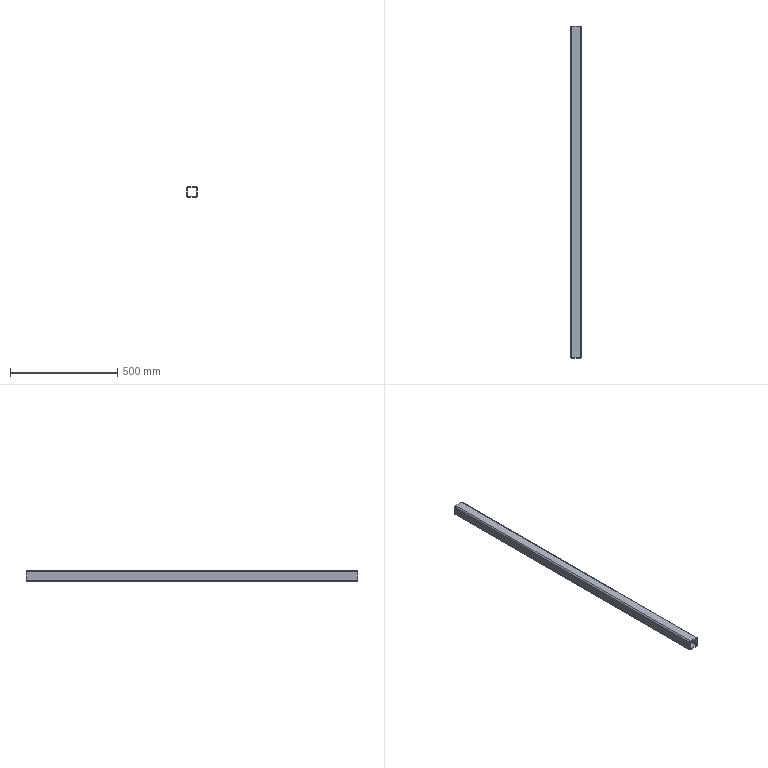Part | SolidWorks | features Extrusion 1 | 1 solid | 18 faces | box 50 x 1550 x 50 mm | volume 1348431 mm3 | plane 10 | cylinder 8 | commonest cylinder face diameters 2 x4 12 x4
STEP:
#1=CARTESIAN_POINT('',(-25.,1550.,19.));
#2=VERTEX_POINT('',#1);
#3=CARTESIAN_POINT('',(-19.,1550.,25.));
#4=VERTEX_POINT('',#3);
#5=CARTESIAN_POINT('',(-19.,1550.,19.));
#6=DIRECTION('',(0.,1.,0.));
#7=DIRECTION('',(0.,0.,-1.));
#8=AXIS2_PLACEMENT_3D('',#5,#6,#7);
#9=CIRCLE('',#8,6.);
#10=EDGE_CURVE('',#2,#4,#9,.T.);
#11=ORIENTED_EDGE('',*,*,#10,.T.);
#12=CARTESIAN_POINT('',(19.,1550.,25.));
#13=VERTEX_POINT('',#12);
#14=CARTESIAN_POINT('',(-19.,1550.,25.));
#15=DIRECTION('',(1.,0.,0.));
#16=VECTOR('',#15,1000.);
#17=LINE('',#14,#16);
#18=EDGE_CURVE('',#4,#13,#17,.T.);
#19=ORIENTED_EDGE('',*,*,#18,.T.);
#20=CARTESIAN_POINT('',(25.,1550.,19.));
#21=VERTEX_POINT('',#20);
#22=CARTESIAN_POINT('',(19.,1550.,19.));
#23=DIRECTION('',(0.,1.,0.));
#24=DIRECTION('',(0.,0.,1.));
#25=AXIS2_PLACEMENT_3D('',#22,#23,#24);
#26=CIRCLE('',#25,6.);
#27=EDGE_CURVE('',#13,#21,#26,.T.);
#28=ORIENTED_EDGE('',*,*,#27,.T.);
#29=CARTESIAN_POINT('',(25.,1550.,-19.));
#30=VERTEX_POINT('',#29);
#31=CARTESIAN_POINT('',(25.,1550.,19.));
#32=DIRECTION('',(0.,0.,-1.));
#33=VECTOR('',#32,1000.);
#34=LINE('',#31,#33);
#35=EDGE_CURVE('',#21,#30,#34,.T.);
#36=ORIENTED_EDGE('',*,*,#35,.T.);
#37=CARTESIAN_POINT('',(19.,1550.,-25.));
#38=VERTEX_POINT('',#37);
#39=CARTESIAN_POINT('',(19.,1550.,-19.));
#40=DIRECTION('',(0.,1.,0.));
#41=DIRECTION('',(0.,0.,-1.));
#42=AXIS2_PLACEMENT_3D('',#39,#40,#41);
#43=CIRCLE('',#42,6.);
#44=EDGE_CURVE('',#30,#38,#43,.T.);
#45=ORIENTED_EDGE('',*,*,#44,.T.);
#46=CARTESIAN_POINT('',(-19.,1550.,-25.));
#47=VERTEX_POINT('',#46);
#48=CARTESIAN_POINT('',(-19.,1550.,-25.));
#49=DIRECTION('',(-1.,0.,0.));
#50=VECTOR('',#49,1000.);
#51=LINE('',#48,#50);
#52=EDGE_CURVE('',#38,#47,#51,.T.);
#53=ORIENTED_EDGE('',*,*,#52,.T.);
#54=CARTESIAN_POINT('',(-25.,1550.,-19.));
#55=VERTEX_POINT('',#54);
#56=CARTESIAN_POINT('',(-19.,1550.,-19.));
#57=DIRECTION('',(0.,1.,0.));
#58=DIRECTION('',(0.,0.,-1.));
#59=AXIS2_PLACEMENT_3D('',#56,#57,#58);
#60=CIRCLE('',#59,6.);
#61=EDGE_CURVE('',#47,#55,#60,.T.);
#62=ORIENTED_EDGE('',*,*,#61,.T.);
#63=CARTESIAN_POINT('',(-25.,1550.,19.));
#64=DIRECTION('',(0.,0.,1.));
#65=VECTOR('',#64,1000.);
#66=LINE('',#63,#65);
#67=EDGE_CURVE('',#55,#2,#66,.T.);
#68=ORIENTED_EDGE('',*,*,#67,.T.);
#69=EDGE_LOOP('',(#11,#19,#28,#36,#45,#53,#62,#68));
#70=FACE_OUTER_BOUND('',#69,.T.);
#71=CARTESIAN_POINT('',(-20.,1550.,19.));
#72=VERTEX_POINT('',#71);
#73=CARTESIAN_POINT('',(-19.,1550.,20.));
#74=VERTEX_POINT('',#73);
#75=CARTESIAN_POINT('',(-19.,1550.,19.));
#76=DIRECTION('',(0.,1.,0.));
#77=DIRECTION('',(0.,0.,-1.));
#78=AXIS2_PLACEMENT_3D('',#75,#76,#77);
#79=CIRCLE('',#78,1.);
#80=EDGE_CURVE('',#72,#74,#79,.T.);
#81=ORIENTED_EDGE('',*,*,#80,.F.);
#82=CARTESIAN_POINT('',(-20.,1550.,-19.));
#83=VERTEX_POINT('',#82);
#84=CARTESIAN_POINT('',(-20.,1550.,19.));
#85=DIRECTION('',(0.,0.,1.));
#86=VECTOR('',#85,1000.);
#87=LINE('',#84,#86);
#88=EDGE_CURVE('',#83,#72,#87,.T.);
#89=ORIENTED_EDGE('',*,*,#88,.F.);
#90=CARTESIAN_POINT('',(-19.,1550.,-20.));
#91=VERTEX_POINT('',#90);
#92=CARTESIAN_POINT('',(-19.,1550.,-19.));
#93=DIRECTION('',(0.,1.,0.));
#94=DIRECTION('',(0.,0.,-1.));
#95=AXIS2_PLACEMENT_3D('',#92,#93,#94);
#96=CIRCLE('',#95,1.);
#97=EDGE_CURVE('',#91,#83,#96,.T.);
#98=ORIENTED_EDGE('',*,*,#97,.F.);
#99=CARTESIAN_POINT('',(19.,1550.,-20.));
#100=VERTEX_POINT('',#99);
#101=CARTESIAN_POINT('',(-19.,1550.,-20.));
#102=DIRECTION('',(-1.,0.,0.));
#103=VECTOR('',#102,1000.);
#104=LINE('',#101,#103);
#105=EDGE_CURVE('',#100,#91,#104,.T.);
#106=ORIENTED_EDGE('',*,*,#105,.F.);
#107=CARTESIAN_POINT('',(20.,1550.,-19.));
#108=VERTEX_POINT('',#107);
#109=CARTESIAN_POINT('',(19.,1550.,-19.));
#110=DIRECTION('',(0.,1.,0.));
#111=DIRECTION('',(0.,0.,-1.));
#112=AXIS2_PLACEMENT_3D('',#109,#110,#111);
#113=CIRCLE('',#112,1.);
#114=EDGE_CURVE('',#108,#100,#113,.T.);
#115=ORIENTED_EDGE('',*,*,#114,.F.);
#116=CARTESIAN_POINT('',(20.,1550.,19.));
#117=VERTEX_POINT('',#116);
#118=CARTESIAN_POINT('',(20.,1550.,19.));
#119=DIRECTION('',(0.,0.,-1.));
#120=VECTOR('',#119,1000.);
#121=LINE('',#118,#120);
#122=EDGE_CURVE('',#117,#108,#121,.T.);
#123=ORIENTED_EDGE('',*,*,#122,.F.);
#124=CARTESIAN_POINT('',(19.,1550.,20.));
#125=VERTEX_POINT('',#124);
#126=CARTESIAN_POINT('',(19.,1550.,19.));
#127=DIRECTION('',(0.,1.,0.));
#128=DIRECTION('',(0.,0.,1.));
#129=AXIS2_PLACEMENT_3D('',#126,#127,#128);
#130=CIRCLE('',#129,1.);
#131=EDGE_CURVE('',#125,#117,#130,.T.);
#132=ORIENTED_EDGE('',*,*,#131,.F.);
#133=CARTESIAN_POINT('',(-19.,1550.,20.));
#134=DIRECTION('',(1.,0.,0.));
#135=VECTOR('',#134,1000.);
#136=LINE('',#133,#135);
#137=EDGE_CURVE('',#74,#125,#136,.T.);
#138=ORIENTED_EDGE('',*,*,#137,.F.);
#139=EDGE_LOOP('',(#81,#89,#98,#106,#115,#123,#132,#138));
#140=FACE_BOUND('',#139,.T.);
#141=CARTESIAN_POINT('',(-19.,1550.,19.));
#142=DIRECTION('',(0.,-1.,0.));
#143=DIRECTION('',(0.,0.,-1.));
#144=AXIS2_PLACEMENT_3D('',#141,#142,#143);
#145=PLANE('',#144);
#146=ADVANCED_FACE('',(#70,#140),#145,.F.);
#147=CARTESIAN_POINT('',(-25.,0.,19.));
#148=VERTEX_POINT('',#147);
#149=CARTESIAN_POINT('',(-19.,0.,25.));
#150=VERTEX_POINT('',#149);
#151=CARTESIAN_POINT('',(-19.,0.,19.));
#152=DIRECTION('',(0.,1.,0.));
#153=DIRECTION('',(0.,0.,-1.));
#154=AXIS2_PLACEMENT_3D('',#151,#152,#153);
#155=CIRCLE('',#154,6.);
#156=EDGE_CURVE('',#148,#150,#155,.T.);
#157=ORIENTED_EDGE('',*,*,#156,.F.);
#158=CARTESIAN_POINT('',(-25.,0.,-19.));
#159=VERTEX_POINT('',#158);
#160=CARTESIAN_POINT('',(-25.,0.,19.));
#161=DIRECTION('',(0.,0.,1.));
#162=VECTOR('',#161,1000.);
#163=LINE('',#160,#162);
#164=EDGE_CURVE('',#159,#148,#163,.T.);
#165=ORIENTED_EDGE('',*,*,#164,.F.);
#166=CARTESIAN_POINT('',(-19.,0.,-25.));
#167=VERTEX_POINT('',#166);
#168=CARTESIAN_POINT('',(-19.,0.,-19.));
#169=DIRECTION('',(0.,1.,0.));
#170=DIRECTION('',(0.,0.,-1.));
#171=AXIS2_PLACEMENT_3D('',#168,#169,#170);
#172=CIRCLE('',#171,6.);
#173=EDGE_CURVE('',#167,#159,#172,.T.);
#174=ORIENTED_EDGE('',*,*,#173,.F.);
#175=CARTESIAN_POINT('',(19.,0.,-25.));
#176=VERTEX_POINT('',#175);
#177=CARTESIAN_POINT('',(-19.,0.,-25.));
#178=DIRECTION('',(-1.,0.,0.));
#179=VECTOR('',#178,1000.);
#180=LINE('',#177,#179);
#181=EDGE_CURVE('',#176,#167,#180,.T.);
#182=ORIENTED_EDGE('',*,*,#181,.F.);
#183=CARTESIAN_POINT('',(25.,0.,-19.));
#184=VERTEX_POINT('',#183);
#185=CARTESIAN_POINT('',(19.,0.,-19.));
#186=DIRECTION('',(0.,1.,0.));
#187=DIRECTION('',(0.,0.,-1.));
#188=AXIS2_PLACEMENT_3D('',#185,#186,#187);
#189=CIRCLE('',#188,6.);
#190=EDGE_CURVE('',#184,#176,#189,.T.);
#191=ORIENTED_EDGE('',*,*,#190,.F.);
#192=CARTESIAN_POINT('',(25.,0.,19.));
#193=VERTEX_POINT('',#192);
#194=CARTESIAN_POINT('',(25.,0.,19.));
#195=DIRECTION('',(0.,0.,-1.));
#196=VECTOR('',#195,1000.);
#197=LINE('',#194,#196);
#198=EDGE_CURVE('',#193,#184,#197,.T.);
#199=ORIENTED_EDGE('',*,*,#198,.F.);
#200=CARTESIAN_POINT('',(19.,0.,25.));
#201=VERTEX_POINT('',#200);
#202=CARTESIAN_POINT('',(19.,0.,19.));
#203=DIRECTION('',(0.,1.,0.));
#204=DIRECTION('',(0.,0.,1.));
#205=AXIS2_PLACEMENT_3D('',#202,#203,#204);
#206=CIRCLE('',#205,6.);
#207=EDGE_CURVE('',#201,#193,#206,.T.);
#208=ORIENTED_EDGE('',*,*,#207,.F.);
#209=CARTESIAN_POINT('',(-19.,0.,25.));
#210=DIRECTION('',(1.,0.,0.));
#211=VECTOR('',#210,1000.);
#212=LINE('',#209,#211);
#213=EDGE_CURVE('',#150,#201,#212,.T.);
#214=ORIENTED_EDGE('',*,*,#213,.F.);
#215=EDGE_LOOP('',(#157,#165,#174,#182,#191,#199,#208,#214));
#216=FACE_OUTER_BOUND('',#215,.T.);
#217=CARTESIAN_POINT('',(-20.,0.,-19.));
#218=VERTEX_POINT('',#217);
#219=CARTESIAN_POINT('',(-20.,0.,19.));
#220=VERTEX_POINT('',#219);
#221=CARTESIAN_POINT('',(-20.,0.,19.));
#222=DIRECTION('',(0.,0.,1.));
#223=VECTOR('',#222,1000.);
#224=LINE('',#221,#223);
#225=EDGE_CURVE('',#218,#220,#224,.T.);
#226=ORIENTED_EDGE('',*,*,#225,.T.);
#227=CARTESIAN_POINT('',(-19.,0.,20.));
#228=VERTEX_POINT('',#227);
#229=CARTESIAN_POINT('',(-19.,0.,19.));
#230=DIRECTION('',(0.,1.,0.));
#231=DIRECTION('',(0.,0.,-1.));
#232=AXIS2_PLACEMENT_3D('',#229,#230,#231);
#233=CIRCLE('',#232,1.);
#234=EDGE_CURVE('',#220,#228,#233,.T.);
#235=ORIENTED_EDGE('',*,*,#234,.T.);
#236=CARTESIAN_POINT('',(19.,0.,20.));
#237=VERTEX_POINT('',#236);
#238=CARTESIAN_POINT('',(-19.,0.,20.));
#239=DIRECTION('',(1.,0.,0.));
#240=VECTOR('',#239,1000.);
#241=LINE('',#238,#240);
#242=EDGE_CURVE('',#228,#237,#241,.T.);
#243=ORIENTED_EDGE('',*,*,#242,.T.);
#244=CARTESIAN_POINT('',(20.,0.,19.));
#245=VERTEX_POINT('',#244);
#246=CARTESIAN_POINT('',(19.,0.,19.));
#247=DIRECTION('',(0.,1.,0.));
#248=DIRECTION('',(0.,0.,1.));
#249=AXIS2_PLACEMENT_3D('',#246,#247,#248);
#250=CIRCLE('',#249,1.);
#251=EDGE_CURVE('',#237,#245,#250,.T.);
#252=ORIENTED_EDGE('',*,*,#251,.T.);
#253=CARTESIAN_POINT('',(20.,0.,-19.));
#254=VERTEX_POINT('',#253);
#255=CARTESIAN_POINT('',(20.,0.,19.));
#256=DIRECTION('',(0.,0.,-1.));
#257=VECTOR('',#256,1000.);
#258=LINE('',#255,#257);
#259=EDGE_CURVE('',#245,#254,#258,.T.);
#260=ORIENTED_EDGE('',*,*,#259,.T.);
#261=CARTESIAN_POINT('',(19.,0.,-20.));
#262=VERTEX_POINT('',#261);
#263=CARTESIAN_POINT('',(19.,0.,-19.));
#264=DIRECTION('',(0.,1.,0.));
#265=DIRECTION('',(0.,0.,-1.));
#266=AXIS2_PLACEMENT_3D('',#263,#264,#265);
#267=CIRCLE('',#266,1.);
#268=EDGE_CURVE('',#254,#262,#267,.T.);
#269=ORIENTED_EDGE('',*,*,#268,.T.);
#270=CARTESIAN_POINT('',(-19.,0.,-20.));
#271=VERTEX_POINT('',#270);
#272=CARTESIAN_POINT('',(-19.,0.,-20.));
#273=DIRECTION('',(-1.,0.,0.));
#274=VECTOR('',#273,1000.);
#275=LINE('',#272,#274);
#276=EDGE_CURVE('',#262,#271,#275,.T.);
#277=ORIENTED_EDGE('',*,*,#276,.T.);
#278=CARTESIAN_POINT('',(-19.,0.,-19.));
#279=DIRECTION('',(0.,1.,0.));
#280=DIRECTION('',(0.,0.,-1.));
#281=AXIS2_PLACEMENT_3D('',#278,#279,#280);
#282=CIRCLE('',#281,1.);
#283=EDGE_CURVE('',#271,#218,#282,.T.);
#284=ORIENTED_EDGE('',*,*,#283,.T.);
#285=EDGE_LOOP('',(#226,#235,#243,#252,#260,#269,#277,#284));
#286=FACE_BOUND('',#285,.T.);
#287=CARTESIAN_POINT('',(-19.,0.,19.));
#288=DIRECTION('',(0.,-1.,0.));
#289=DIRECTION('',(0.,0.,-1.));
#290=AXIS2_PLACEMENT_3D('',#287,#288,#289);
#291=PLANE('',#290);
#292=ADVANCED_FACE('',(#216,#286),#291,.T.);
#293=ORIENTED_EDGE('',*,*,#156,.T.);
#294=CARTESIAN_POINT('',(-19.,1550.,25.));
#295=DIRECTION('',(0.,-1.,0.));
#296=VECTOR('',#295,1000.);
#297=LINE('',#294,#296);
#298=EDGE_CURVE('',#4,#150,#297,.T.);
#299=ORIENTED_EDGE('',*,*,#298,.F.);
#300=ORIENTED_EDGE('',*,*,#10,.F.);
#301=CARTESIAN_POINT('',(-25.,1550.,19.));
#302=DIRECTION('',(0.,-1.,0.));
#303=VECTOR('',#302,1000.);
#304=LINE('',#301,#303);
#305=EDGE_CURVE('',#2,#148,#304,.T.);
#306=ORIENTED_EDGE('',*,*,#305,.T.);
#307=EDGE_LOOP('',(#293,#299,#300,#306));
#308=FACE_OUTER_BOUND('',#307,.T.);
#309=CARTESIAN_POINT('',(-19.,1550.,19.));
#310=DIRECTION('',(0.,-1.,0.));
#311=DIRECTION('',(0.,0.,-1.));
#312=AXIS2_PLACEMENT_3D('',#309,#310,#311);
#313=CYLINDRICAL_SURFACE('',#312,6.);
#314=ADVANCED_FACE('',(#308),#313,.T.);
#315=ORIENTED_EDGE('',*,*,#213,.T.);
#316=CARTESIAN_POINT('',(19.,1550.,25.));
#317=DIRECTION('',(0.,-1.,0.));
#318=VECTOR('',#317,1000.);
#319=LINE('',#316,#318);
#320=EDGE_CURVE('',#13,#201,#319,.T.);
#321=ORIENTED_EDGE('',*,*,#320,.F.);
#322=ORIENTED_EDGE('',*,*,#18,.F.);
#323=ORIENTED_EDGE('',*,*,#298,.T.);
#324=EDGE_LOOP('',(#315,#321,#322,#323));
#325=FACE_OUTER_BOUND('',#324,.T.);
#326=CARTESIAN_POINT('',(-19.,1550.,25.));
#327=DIRECTION('',(0.,0.,-1.));
#328=DIRECTION('',(-1.,0.,0.));
#329=AXIS2_PLACEMENT_3D('',#326,#327,#328);
#330=PLANE('',#329);
#331=ADVANCED_FACE('',(#325),#330,.F.);
#332=ORIENTED_EDGE('',*,*,#207,.T.);
#333=CARTESIAN_POINT('',(25.,1550.,19.));
#334=DIRECTION('',(0.,-1.,0.));
#335=VECTOR('',#334,1000.);
#336=LINE('',#333,#335);
#337=EDGE_CURVE('',#21,#193,#336,.T.);
#338=ORIENTED_EDGE('',*,*,#337,.F.);
#339=ORIENTED_EDGE('',*,*,#27,.F.);
#340=ORIENTED_EDGE('',*,*,#320,.T.);
#341=EDGE_LOOP('',(#332,#338,#339,#340));
#342=FACE_OUTER_BOUND('',#341,.T.);
#343=CARTESIAN_POINT('',(19.,1550.,19.));
#344=DIRECTION('',(0.,-1.,0.));
#345=DIRECTION('',(0.,0.,-1.));
#346=AXIS2_PLACEMENT_3D('',#343,#344,#345);
#347=CYLINDRICAL_SURFACE('',#346,6.);
#348=ADVANCED_FACE('',(#342),#347,.T.);
#349=ORIENTED_EDGE('',*,*,#198,.T.);
#350=CARTESIAN_POINT('',(25.,1550.,-19.));
#351=DIRECTION('',(0.,-1.,0.));
#352=VECTOR('',#351,1000.);
#353=LINE('',#350,#352);
#354=EDGE_CURVE('',#30,#184,#353,.T.);
#355=ORIENTED_EDGE('',*,*,#354,.F.);
#356=ORIENTED_EDGE('',*,*,#35,.F.);
#357=ORIENTED_EDGE('',*,*,#337,.T.);
#358=EDGE_LOOP('',(#349,#355,#356,#357));
#359=FACE_OUTER_BOUND('',#358,.T.);
#360=CARTESIAN_POINT('',(25.,1550.,19.));
#361=DIRECTION('',(-1.,0.,0.));
#362=DIRECTION('',(0.,0.,1.));
#363=AXIS2_PLACEMENT_3D('',#360,#361,#362);
#364=PLANE('',#363);
#365=ADVANCED_FACE('',(#359),#364,.F.);
#366=ORIENTED_EDGE('',*,*,#190,.T.);
#367=CARTESIAN_POINT('',(19.,1550.,-25.));
#368=DIRECTION('',(0.,-1.,0.));
#369=VECTOR('',#368,1000.);
#370=LINE('',#367,#369);
#371=EDGE_CURVE('',#38,#176,#370,.T.);
#372=ORIENTED_EDGE('',*,*,#371,.F.);
#373=ORIENTED_EDGE('',*,*,#44,.F.);
#374=ORIENTED_EDGE('',*,*,#354,.T.);
#375=EDGE_LOOP('',(#366,#372,#373,#374));
#376=FACE_OUTER_BOUND('',#375,.T.);
#377=CARTESIAN_POINT('',(19.,1550.,-19.));
#378=DIRECTION('',(0.,-1.,0.));
#379=DIRECTION('',(0.,0.,-1.));
#380=AXIS2_PLACEMENT_3D('',#377,#378,#379);
#381=CYLINDRICAL_SURFACE('',#380,6.);
#382=ADVANCED_FACE('',(#376),#381,.T.);
#383=ORIENTED_EDGE('',*,*,#181,.T.);
#384=CARTESIAN_POINT('',(-19.,1550.,-25.));
#385=DIRECTION('',(0.,-1.,0.));
#386=VECTOR('',#385,1000.);
#387=LINE('',#384,#386);
#388=EDGE_CURVE('',#47,#167,#387,.T.);
#389=ORIENTED_EDGE('',*,*,#388,.F.);
#390=ORIENTED_EDGE('',*,*,#52,.F.);
#391=ORIENTED_EDGE('',*,*,#371,.T.);
#392=EDGE_LOOP('',(#383,#389,#390,#391));
#393=FACE_OUTER_BOUND('',#392,.T.);
#394=CARTESIAN_POINT('',(-19.,1550.,-25.));
#395=DIRECTION('',(0.,0.,1.));
#396=DIRECTION('',(1.,0.,0.));
#397=AXIS2_PLACEMENT_3D('',#394,#395,#396);
#398=PLANE('',#397);
#399=ADVANCED_FACE('',(#393),#398,.F.);
#400=ORIENTED_EDGE('',*,*,#173,.T.);
#401=CARTESIAN_POINT('',(-25.,1550.,-19.));
#402=DIRECTION('',(0.,-1.,0.));
#403=VECTOR('',#402,1000.);
#404=LINE('',#401,#403);
#405=EDGE_CURVE('',#55,#159,#404,.T.);
#406=ORIENTED_EDGE('',*,*,#405,.F.);
#407=ORIENTED_EDGE('',*,*,#61,.F.);
#408=ORIENTED_EDGE('',*,*,#388,.T.);
#409=EDGE_LOOP('',(#400,#406,#407,#408));
#410=FACE_OUTER_BOUND('',#409,.T.);
#411=CARTESIAN_POINT('',(-19.,1550.,-19.));
#412=DIRECTION('',(0.,-1.,0.));
#413=DIRECTION('',(0.,0.,-1.));
#414=AXIS2_PLACEMENT_3D('',#411,#412,#413);
#415=CYLINDRICAL_SURFACE('',#414,6.);
#416=ADVANCED_FACE('',(#410),#415,.T.);
#417=ORIENTED_EDGE('',*,*,#164,.T.);
#418=ORIENTED_EDGE('',*,*,#305,.F.);
#419=ORIENTED_EDGE('',*,*,#67,.F.);
#420=ORIENTED_EDGE('',*,*,#405,.T.);
#421=EDGE_LOOP('',(#417,#418,#419,#420));
#422=FACE_OUTER_BOUND('',#421,.T.);
#423=CARTESIAN_POINT('',(-25.,1550.,19.));
#424=DIRECTION('',(1.,0.,0.));
#425=DIRECTION('',(0.,0.,-1.));
#426=AXIS2_PLACEMENT_3D('',#423,#424,#425);
#427=PLANE('',#426);
#428=ADVANCED_FACE('',(#422),#427,.F.);
#429=ORIENTED_EDGE('',*,*,#234,.F.);
#430=CARTESIAN_POINT('',(-20.,1550.,19.));
#431=DIRECTION('',(0.,-1.,0.));
#432=VECTOR('',#431,1000.);
#433=LINE('',#430,#432);
#434=EDGE_CURVE('',#72,#220,#433,.T.);
#435=ORIENTED_EDGE('',*,*,#434,.F.);
#436=ORIENTED_EDGE('',*,*,#80,.T.);
#437=CARTESIAN_POINT('',(-19.,1550.,20.));
#438=DIRECTION('',(0.,-1.,0.));
#439=VECTOR('',#438,1000.);
#440=LINE('',#437,#439);
#441=EDGE_CURVE('',#74,#228,#440,.T.);
#442=ORIENTED_EDGE('',*,*,#441,.T.);
#443=EDGE_LOOP('',(#429,#435,#436,#442));
#444=FACE_OUTER_BOUND('',#443,.T.);
#445=CARTESIAN_POINT('',(-19.,1550.,19.));
#446=DIRECTION('',(0.,-1.,0.));
#447=DIRECTION('',(0.,0.,-1.));
#448=AXIS2_PLACEMENT_3D('',#445,#446,#447);
#449=CYLINDRICAL_SURFACE('',#448,1.);
#450=ADVANCED_FACE('',(#444),#449,.F.);
#451=ORIENTED_EDGE('',*,*,#242,.F.);
#452=ORIENTED_EDGE('',*,*,#441,.F.);
#453=ORIENTED_EDGE('',*,*,#137,.T.);
#454=CARTESIAN_POINT('',(19.,1550.,20.));
#455=DIRECTION('',(0.,-1.,0.));
#456=VECTOR('',#455,1000.);
#457=LINE('',#454,#456);
#458=EDGE_CURVE('',#125,#237,#457,.T.);
#459=ORIENTED_EDGE('',*,*,#458,.T.);
#460=EDGE_LOOP('',(#451,#452,#453,#459));
#461=FACE_OUTER_BOUND('',#460,.T.);
#462=CARTESIAN_POINT('',(-19.,1550.,20.));
#463=DIRECTION('',(0.,0.,-1.));
#464=DIRECTION('',(-1.,0.,0.));
#465=AXIS2_PLACEMENT_3D('',#462,#463,#464);
#466=PLANE('',#465);
#467=ADVANCED_FACE('',(#461),#466,.T.);
#468=ORIENTED_EDGE('',*,*,#251,.F.);
#469=ORIENTED_EDGE('',*,*,#458,.F.);
#470=ORIENTED_EDGE('',*,*,#131,.T.);
#471=CARTESIAN_POINT('',(20.,1550.,19.));
#472=DIRECTION('',(0.,-1.,0.));
#473=VECTOR('',#472,1000.);
#474=LINE('',#471,#473);
#475=EDGE_CURVE('',#117,#245,#474,.T.);
#476=ORIENTED_EDGE('',*,*,#475,.T.);
#477=EDGE_LOOP('',(#468,#469,#470,#476));
#478=FACE_OUTER_BOUND('',#477,.T.);
#479=CARTESIAN_POINT('',(19.,1550.,19.));
#480=DIRECTION('',(0.,-1.,0.));
#481=DIRECTION('',(0.,0.,-1.));
#482=AXIS2_PLACEMENT_3D('',#479,#480,#481);
#483=CYLINDRICAL_SURFACE('',#482,1.);
#484=ADVANCED_FACE('',(#478),#483,.F.);
#485=ORIENTED_EDGE('',*,*,#259,.F.);
#486=ORIENTED_EDGE('',*,*,#475,.F.);
#487=ORIENTED_EDGE('',*,*,#122,.T.);
#488=CARTESIAN_POINT('',(20.,1550.,-19.));
#489=DIRECTION('',(0.,-1.,0.));
#490=VECTOR('',#489,1000.);
#491=LINE('',#488,#490);
#492=EDGE_CURVE('',#108,#254,#491,.T.);
#493=ORIENTED_EDGE('',*,*,#492,.T.);
#494=EDGE_LOOP('',(#485,#486,#487,#493));
#495=FACE_OUTER_BOUND('',#494,.T.);
#496=CARTESIAN_POINT('',(20.,1550.,19.));
#497=DIRECTION('',(-1.,0.,0.));
#498=DIRECTION('',(0.,0.,1.));
#499=AXIS2_PLACEMENT_3D('',#496,#497,#498);
#500=PLANE('',#499);
#501=ADVANCED_FACE('',(#495),#500,.T.);
#502=ORIENTED_EDGE('',*,*,#268,.F.);
#503=ORIENTED_EDGE('',*,*,#492,.F.);
#504=ORIENTED_EDGE('',*,*,#114,.T.);
#505=CARTESIAN_POINT('',(19.,1550.,-20.));
#506=DIRECTION('',(0.,-1.,0.));
#507=VECTOR('',#506,1000.);
#508=LINE('',#505,#507);
#509=EDGE_CURVE('',#100,#262,#508,.T.);
#510=ORIENTED_EDGE('',*,*,#509,.T.);
#511=EDGE_LOOP('',(#502,#503,#504,#510));
#512=FACE_OUTER_BOUND('',#511,.T.);
#513=CARTESIAN_POINT('',(19.,1550.,-19.));
#514=DIRECTION('',(0.,-1.,0.));
#515=DIRECTION('',(0.,0.,-1.));
#516=AXIS2_PLACEMENT_3D('',#513,#514,#515);
#517=CYLINDRICAL_SURFACE('',#516,1.);
#518=ADVANCED_FACE('',(#512),#517,.F.);
#519=ORIENTED_EDGE('',*,*,#276,.F.);
#520=ORIENTED_EDGE('',*,*,#509,.F.);
#521=ORIENTED_EDGE('',*,*,#105,.T.);
#522=CARTESIAN_POINT('',(-19.,1550.,-20.));
#523=DIRECTION('',(0.,-1.,0.));
#524=VECTOR('',#523,1000.);
#525=LINE('',#522,#524);
#526=EDGE_CURVE('',#91,#271,#525,.T.);
#527=ORIENTED_EDGE('',*,*,#526,.T.);
#528=EDGE_LOOP('',(#519,#520,#521,#527));
#529=FACE_OUTER_BOUND('',#528,.T.);
#530=CARTESIAN_POINT('',(-19.,1550.,-20.));
#531=DIRECTION('',(0.,0.,1.));
#532=DIRECTION('',(1.,0.,0.));
#533=AXIS2_PLACEMENT_3D('',#530,#531,#532);
#534=PLANE('',#533);
#535=ADVANCED_FACE('',(#529),#534,.T.);
#536=ORIENTED_EDGE('',*,*,#283,.F.);
#537=ORIENTED_EDGE('',*,*,#526,.F.);
#538=ORIENTED_EDGE('',*,*,#97,.T.);
#539=CARTESIAN_POINT('',(-20.,1550.,-19.));
#540=DIRECTION('',(0.,-1.,0.));
#541=VECTOR('',#540,1000.);
#542=LINE('',#539,#541);
#543=EDGE_CURVE('',#83,#218,#542,.T.);
#544=ORIENTED_EDGE('',*,*,#543,.T.);
#545=EDGE_LOOP('',(#536,#537,#538,#544));
#546=FACE_OUTER_BOUND('',#545,.T.);
#547=CARTESIAN_POINT('',(-19.,1550.,-19.));
#548=DIRECTION('',(0.,-1.,0.));
#549=DIRECTION('',(0.,0.,-1.));
#550=AXIS2_PLACEMENT_3D('',#547,#548,#549);
#551=CYLINDRICAL_SURFACE('',#550,1.);
#552=ADVANCED_FACE('',(#546),#551,.F.);
#553=ORIENTED_EDGE('',*,*,#225,.F.);
#554=ORIENTED_EDGE('',*,*,#543,.F.);
#555=ORIENTED_EDGE('',*,*,#88,.T.);
#556=ORIENTED_EDGE('',*,*,#434,.T.);
#557=EDGE_LOOP('',(#553,#554,#555,#556));
#558=FACE_OUTER_BOUND('',#557,.T.);
#559=CARTESIAN_POINT('',(-20.,1550.,19.));
#560=DIRECTION('',(1.,0.,0.));
#561=DIRECTION('',(0.,0.,-1.));
#562=AXIS2_PLACEMENT_3D('',#559,#560,#561);
#563=PLANE('',#562);
#564=ADVANCED_FACE('',(#558),#563,.T.);
#565=CLOSED_SHELL('',(#146,#292,#314,#331,#348,#365,#382,#399,#416,#428,#450,#467,#484,#501,#518,#535,#552,#564));
#566=MANIFOLD_SOLID_BREP('',#565);
#567=CARTESIAN_POINT('',(0.,0.,0.));
#568=DIRECTION('',(0.,0.,1.));
#569=DIRECTION('',(1.,0.,0.));
#570=AXIS2_PLACEMENT_3D('',#567,#568,#569);
#571=(LENGTH_UNIT()NAMED_UNIT(*)SI_UNIT(.MILLI.,.METRE.));
#572=UNCERTAINTY_MEASURE_WITH_UNIT(LENGTH_MEASURE(0.00001),#571,'','');
#573=(NAMED_UNIT(*)PLANE_ANGLE_UNIT()SI_UNIT($,.RADIAN.));
#574=(NAMED_UNIT(*)SI_UNIT($,.STERADIAN.)SOLID_ANGLE_UNIT());
#575=(GEOMETRIC_REPRESENTATION_CONTEXT(3)GLOBAL_UNCERTAINTY_ASSIGNED_CONTEXT((#572))GLOBAL_UNIT_ASSIGNED_CONTEXT((#571,#573,#574))REPRESENTATION_CONTEXT('',''));
#576=ADVANCED_BREP_SHAPE_REPRESENTATION('',(#566,#570),#575);